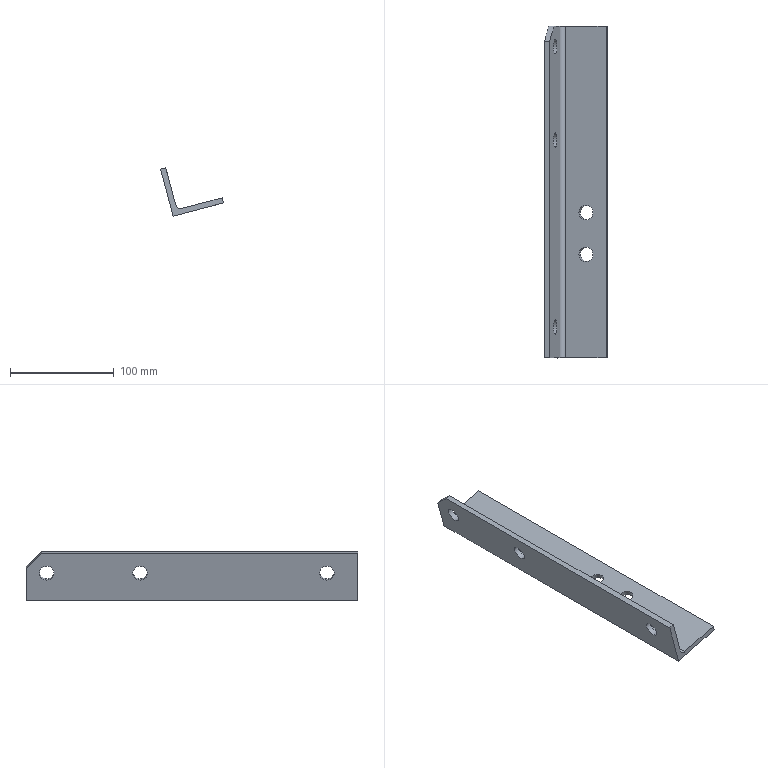Part | NX | features solid 2 | 1 solid | 15 faces | box 60.461 x 320 x 46.693 mm | volume 144506 mm3 | plane 9 | cylinder 6 | commonest cylinder face diameters 14 x5 10 x1
STEP:
#1=CARTESIAN_POINT('',(712.611,850.,-13.897));
#2=VERTEX_POINT('',#1);
#3=CARTESIAN_POINT('',(719.373,850.,-12.085));
#4=DIRECTION('',(-0.2588,0.,0.9659));
#5=DIRECTION('',(-0.9659,0.,-0.2588));
#6=AXIS2_PLACEMENT_3D('',#3,#4,#5);
#7=CIRCLE('',#6,7.);
#8=EDGE_CURVE('',#2,#2,#7,.T.);
#9=ORIENTED_EDGE('',*,*,#8,.F.);
#10=EDGE_LOOP('',(#9));
#11=FACE_BOUND('',#10,.T.);
#12=CARTESIAN_POINT('',(712.611,890.,-13.897));
#13=VERTEX_POINT('',#12);
#14=CARTESIAN_POINT('',(719.373,890.,-12.085));
#15=DIRECTION('',(-0.2588,0.,0.9659));
#16=DIRECTION('',(-0.9659,0.,-0.2588));
#17=AXIS2_PLACEMENT_3D('',#14,#15,#16);
#18=CIRCLE('',#17,7.);
#19=EDGE_CURVE('',#13,#13,#18,.T.);
#20=ORIENTED_EDGE('',*,*,#19,.F.);
#21=EDGE_LOOP('',(#20));
#22=FACE_BOUND('',#21,.T.);
#23=CARTESIAN_POINT('',(700.054,1070.,-17.261));
#24=VERTEX_POINT('',#23);
#25=CARTESIAN_POINT('',(700.054,750.,-17.261));
#26=VERTEX_POINT('',#25);
#27=CARTESIAN_POINT('',(700.054,775.,-17.261));
#28=DIRECTION('',(0.,1.,0.));
#29=VECTOR('',#28,1000.);
#30=LINE('',#27,#29);
#31=EDGE_CURVE('',#24,#26,#30,.F.);
#32=ORIENTED_EDGE('',*,*,#31,.T.);
#33=CARTESIAN_POINT('',(738.691,750.,-6.909));
#34=VERTEX_POINT('',#33);
#35=CARTESIAN_POINT('',(738.691,750.,-6.909));
#36=DIRECTION('',(0.9659,0.,0.2588));
#37=VECTOR('',#36,1000.);
#38=LINE('',#35,#37);
#39=EDGE_CURVE('',#26,#34,#38,.T.);
#40=ORIENTED_EDGE('',*,*,#39,.T.);
#41=CARTESIAN_POINT('',(738.691,1070.,-6.909));
#42=VERTEX_POINT('',#41);
#43=CARTESIAN_POINT('',(738.691,894.636,-6.909));
#44=DIRECTION('',(0.,1.,0.));
#45=VECTOR('',#44,1000.);
#46=LINE('',#43,#45);
#47=EDGE_CURVE('',#34,#42,#46,.T.);
#48=ORIENTED_EDGE('',*,*,#47,.T.);
#49=CARTESIAN_POINT('',(738.691,1070.,-6.909));
#50=DIRECTION('',(0.9659,0.,0.2588));
#51=VECTOR('',#50,1000.);
#52=LINE('',#49,#51);
#53=EDGE_CURVE('',#24,#42,#52,.T.);
#54=ORIENTED_EDGE('',*,*,#53,.F.);
#55=EDGE_LOOP('',(#32,#40,#48,#54));
#56=FACE_BOUND('',#55,.T.);
#57=CARTESIAN_POINT('',(738.691,892.805,-6.909));
#58=DIRECTION('',(-0.2588,0.,0.9659));
#59=DIRECTION('',(0.,1.,0.));
#60=AXIS2_PLACEMENT_3D('',#57,#58,#59);
#61=PLANE('',#60);
#62=ADVANCED_FACE('',(#11,#22,#56),#61,.T.);
#63=CARTESIAN_POINT('',(713.905,850.,-18.726));
#64=VERTEX_POINT('',#63);
#65=CARTESIAN_POINT('',(720.667,850.,-16.915));
#66=DIRECTION('',(-0.2588,0.,0.9659));
#67=DIRECTION('',(-0.9659,0.,-0.2588));
#68=AXIS2_PLACEMENT_3D('',#65,#66,#67);
#69=CIRCLE('',#68,7.);
#70=EDGE_CURVE('',#64,#64,#69,.F.);
#71=ORIENTED_EDGE('',*,*,#70,.F.);
#72=EDGE_LOOP('',(#71));
#73=FACE_BOUND('',#72,.T.);
#74=CARTESIAN_POINT('',(713.905,890.,-18.726));
#75=VERTEX_POINT('',#74);
#76=CARTESIAN_POINT('',(720.667,890.,-16.915));
#77=DIRECTION('',(-0.2588,0.,0.9659));
#78=DIRECTION('',(-0.9659,0.,-0.2588));
#79=AXIS2_PLACEMENT_3D('',#76,#77,#78);
#80=CIRCLE('',#79,7.);
#81=EDGE_CURVE('',#75,#75,#80,.F.);
#82=ORIENTED_EDGE('',*,*,#81,.F.);
#83=EDGE_LOOP('',(#82));
#84=FACE_BOUND('',#83,.T.);
#85=CARTESIAN_POINT('',(739.985,750.,-11.738));
#86=VERTEX_POINT('',#85);
#87=CARTESIAN_POINT('',(739.985,1070.,-11.738));
#88=VERTEX_POINT('',#87);
#89=CARTESIAN_POINT('',(739.985,892.5,-11.738));
#90=DIRECTION('',(0.,1.,0.));
#91=VECTOR('',#90,1000.);
#92=LINE('',#89,#91);
#93=EDGE_CURVE('',#86,#88,#92,.T.);
#94=ORIENTED_EDGE('',*,*,#93,.F.);
#95=CARTESIAN_POINT('',(691.689,750.,-24.679));
#96=VERTEX_POINT('',#95);
#97=CARTESIAN_POINT('',(696.519,750.,-23.385));
#98=DIRECTION('',(-0.9659,0.,-0.2588));
#99=VECTOR('',#98,1000.);
#100=LINE('',#97,#99);
#101=EDGE_CURVE('',#86,#96,#100,.T.);
#102=ORIENTED_EDGE('',*,*,#101,.T.);
#103=CARTESIAN_POINT('',(691.689,1070.,-24.679));
#104=VERTEX_POINT('',#103);
#105=CARTESIAN_POINT('',(691.689,894.636,-24.679));
#106=DIRECTION('',(0.,1.,0.));
#107=VECTOR('',#106,1000.);
#108=LINE('',#105,#107);
#109=EDGE_CURVE('',#96,#104,#108,.T.);
#110=ORIENTED_EDGE('',*,*,#109,.T.);
#111=CARTESIAN_POINT('',(696.519,1070.,-23.385));
#112=DIRECTION('',(-0.9659,0.,-0.2588));
#113=VECTOR('',#112,1000.);
#114=LINE('',#111,#113);
#115=EDGE_CURVE('',#88,#104,#114,.T.);
#116=ORIENTED_EDGE('',*,*,#115,.F.);
#117=EDGE_LOOP('',(#94,#102,#110,#116));
#118=FACE_BOUND('',#117,.T.);
#119=CARTESIAN_POINT('',(696.519,892.5,-23.385));
#120=DIRECTION('',(0.2588,0.,-0.9659));
#121=DIRECTION('',(0.,-1.,0.));
#122=AXIS2_PLACEMENT_3D('',#119,#120,#121);
#123=PLANE('',#122);
#124=ADVANCED_FACE('',(#73,#84,#118),#123,.T.);
#125=CARTESIAN_POINT('',(687.719,1050.,9.456));
#126=VERTEX_POINT('',#125);
#127=CARTESIAN_POINT('',(689.531,1050.,2.695));
#128=DIRECTION('',(0.9659,0.,0.2588));
#129=DIRECTION('',(-0.2588,0.,0.9659));
#130=AXIS2_PLACEMENT_3D('',#127,#128,#129);
#131=CIRCLE('',#130,7.);
#132=EDGE_CURVE('',#126,#126,#131,.F.);
#133=ORIENTED_EDGE('',*,*,#132,.T.);
#134=EDGE_LOOP('',(#133));
#135=FACE_BOUND('',#134,.T.);
#136=CARTESIAN_POINT('',(691.342,960.,-4.067));
#137=VERTEX_POINT('',#136);
#138=CARTESIAN_POINT('',(689.531,960.,2.695));
#139=DIRECTION('',(-0.9659,0.,-0.2588));
#140=DIRECTION('',(0.2588,0.,-0.9659));
#141=AXIS2_PLACEMENT_3D('',#138,#139,#140);
#142=CIRCLE('',#141,7.);
#143=EDGE_CURVE('',#137,#137,#142,.F.);
#144=ORIENTED_EDGE('',*,*,#143,.F.);
#145=EDGE_LOOP('',(#144));
#146=FACE_BOUND('',#145,.T.);
#147=CARTESIAN_POINT('',(691.342,780.,-4.067));
#148=VERTEX_POINT('',#147);
#149=CARTESIAN_POINT('',(689.531,780.,2.695));
#150=DIRECTION('',(-0.9659,0.,-0.2588));
#151=DIRECTION('',(0.2588,0.,-0.9659));
#152=AXIS2_PLACEMENT_3D('',#149,#150,#151);
#153=CIRCLE('',#152,7.);
#154=EDGE_CURVE('',#148,#148,#153,.F.);
#155=ORIENTED_EDGE('',*,*,#154,.F.);
#156=EDGE_LOOP('',(#155));
#157=FACE_BOUND('',#156,.T.);
#158=CARTESIAN_POINT('',(684.354,750.,22.013));
#159=VERTEX_POINT('',#158);
#160=CARTESIAN_POINT('',(684.354,1055.,22.013));
#161=VERTEX_POINT('',#160);
#162=CARTESIAN_POINT('',(684.354,894.636,22.013));
#163=DIRECTION('',(0.,1.,0.));
#164=VECTOR('',#163,1000.);
#165=LINE('',#162,#164);
#166=EDGE_CURVE('',#159,#161,#165,.T.);
#167=ORIENTED_EDGE('',*,*,#166,.F.);
#168=CARTESIAN_POINT('',(693.93,750.,-13.726));
#169=VERTEX_POINT('',#168);
#170=CARTESIAN_POINT('',(687.46,750.,10.422));
#171=DIRECTION('',(0.2588,0.,-0.9659));
#172=VECTOR('',#171,1000.);
#173=LINE('',#170,#172);
#174=EDGE_CURVE('',#159,#169,#173,.T.);
#175=ORIENTED_EDGE('',*,*,#174,.T.);
#176=CARTESIAN_POINT('',(693.93,1070.,-13.726));
#177=VERTEX_POINT('',#176);
#178=CARTESIAN_POINT('',(693.93,1109.813,-13.726));
#179=DIRECTION('',(0.,1.,0.));
#180=VECTOR('',#179,1000.);
#181=LINE('',#178,#180);
#182=EDGE_CURVE('',#169,#177,#181,.T.);
#183=ORIENTED_EDGE('',*,*,#182,.T.);
#184=CARTESIAN_POINT('',(688.236,1070.,7.525));
#185=VERTEX_POINT('',#184);
#186=CARTESIAN_POINT('',(687.46,1070.,10.422));
#187=DIRECTION('',(0.2588,0.,-0.9659));
#188=VECTOR('',#187,1000.);
#189=LINE('',#186,#188);
#190=EDGE_CURVE('',#185,#177,#189,.T.);
#191=ORIENTED_EDGE('',*,*,#190,.F.);
#192=CARTESIAN_POINT('',(665.154,980.818,93.668));
#193=DIRECTION('',(-0.183,-0.7071,0.683));
#194=VECTOR('',#193,1000.);
#195=LINE('',#192,#194);
#196=EDGE_CURVE('',#185,#161,#195,.T.);
#197=ORIENTED_EDGE('',*,*,#196,.T.);
#198=EDGE_LOOP('',(#167,#175,#183,#191,#197));
#199=FACE_BOUND('',#198,.T.);
#200=CARTESIAN_POINT('',(687.46,894.636,10.422));
#201=DIRECTION('',(0.9659,0.,0.2588));
#202=DIRECTION('',(0.2588,0.,-0.9659));
#203=AXIS2_PLACEMENT_3D('',#200,#201,#202);
#204=PLANE('',#203);
#205=ADVANCED_FACE('',(#135,#146,#157,#199),#204,.T.);
#206=CARTESIAN_POINT('',(686.513,1050.,-5.361));
#207=VERTEX_POINT('',#206);
#208=CARTESIAN_POINT('',(684.701,1050.,1.401));
#209=DIRECTION('',(-0.9659,0.,-0.2588));
#210=DIRECTION('',(0.2588,0.,-0.9659));
#211=AXIS2_PLACEMENT_3D('',#208,#209,#210);
#212=CIRCLE('',#211,7.);
#213=EDGE_CURVE('',#207,#207,#212,.T.);
#214=ORIENTED_EDGE('',*,*,#213,.F.);
#215=EDGE_LOOP('',(#214));
#216=FACE_BOUND('',#215,.T.);
#217=CARTESIAN_POINT('',(682.889,960.,8.162));
#218=VERTEX_POINT('',#217);
#219=CARTESIAN_POINT('',(684.701,960.,1.401));
#220=DIRECTION('',(0.9659,0.,0.2588));
#221=DIRECTION('',(-0.2588,0.,0.9659));
#222=AXIS2_PLACEMENT_3D('',#219,#220,#221);
#223=CIRCLE('',#222,7.);
#224=EDGE_CURVE('',#218,#218,#223,.F.);
#225=ORIENTED_EDGE('',*,*,#224,.F.);
#226=EDGE_LOOP('',(#225));
#227=FACE_BOUND('',#226,.T.);
#228=CARTESIAN_POINT('',(682.889,780.,8.162));
#229=VERTEX_POINT('',#228);
#230=CARTESIAN_POINT('',(684.701,780.,1.401));
#231=DIRECTION('',(0.9659,0.,0.2588));
#232=DIRECTION('',(-0.2588,0.,0.9659));
#233=AXIS2_PLACEMENT_3D('',#230,#231,#232);
#234=CIRCLE('',#233,7.);
#235=EDGE_CURVE('',#229,#229,#234,.F.);
#236=ORIENTED_EDGE('',*,*,#235,.F.);
#237=EDGE_LOOP('',(#236));
#238=FACE_BOUND('',#237,.T.);
#239=ORIENTED_EDGE('',*,*,#109,.F.);
#240=CARTESIAN_POINT('',(679.525,750.,20.719));
#241=VERTEX_POINT('',#240);
#242=CARTESIAN_POINT('',(682.63,750.,9.128));
#243=DIRECTION('',(-0.2588,0.,0.9659));
#244=VECTOR('',#243,1000.);
#245=LINE('',#242,#244);
#246=EDGE_CURVE('',#96,#241,#245,.T.);
#247=ORIENTED_EDGE('',*,*,#246,.T.);
#248=CARTESIAN_POINT('',(679.525,1055.,20.719));
#249=VERTEX_POINT('',#248);
#250=CARTESIAN_POINT('',(679.525,894.636,20.719));
#251=DIRECTION('',(0.,1.,0.));
#252=VECTOR('',#251,1000.);
#253=LINE('',#250,#252);
#254=EDGE_CURVE('',#241,#249,#253,.T.);
#255=ORIENTED_EDGE('',*,*,#254,.T.);
#256=CARTESIAN_POINT('',(683.407,1070.,6.23));
#257=VERTEX_POINT('',#256);
#258=CARTESIAN_POINT('',(660.325,980.818,92.374));
#259=DIRECTION('',(0.183,0.7071,-0.683));
#260=VECTOR('',#259,1000.);
#261=LINE('',#258,#260);
#262=EDGE_CURVE('',#249,#257,#261,.T.);
#263=ORIENTED_EDGE('',*,*,#262,.T.);
#264=CARTESIAN_POINT('',(682.63,1070.,9.128));
#265=DIRECTION('',(-0.2588,0.,0.9659));
#266=VECTOR('',#265,1000.);
#267=LINE('',#264,#266);
#268=EDGE_CURVE('',#104,#257,#267,.T.);
#269=ORIENTED_EDGE('',*,*,#268,.F.);
#270=EDGE_LOOP('',(#239,#247,#255,#263,#269));
#271=FACE_BOUND('',#270,.T.);
#272=CARTESIAN_POINT('',(682.63,894.636,9.128));
#273=DIRECTION('',(-0.9659,0.,-0.2588));
#274=DIRECTION('',(-0.2588,0.,0.9659));
#275=AXIS2_PLACEMENT_3D('',#272,#273,#274);
#276=PLANE('',#275);
#277=ADVANCED_FACE('',(#216,#227,#238,#271),#276,.T.);
#278=ORIENTED_EDGE('',*,*,#254,.F.);
#279=CARTESIAN_POINT('',(689.184,750.,23.308));
#280=DIRECTION('',(0.9659,0.,0.2588));
#281=VECTOR('',#280,1000.);
#282=LINE('',#279,#281);
#283=EDGE_CURVE('',#241,#159,#282,.T.);
#284=ORIENTED_EDGE('',*,*,#283,.T.);
#285=ORIENTED_EDGE('',*,*,#166,.T.);
#286=CARTESIAN_POINT('',(679.525,1055.,20.719));
#287=DIRECTION('',(-0.9659,0.,-0.2588));
#288=VECTOR('',#287,1000.);
#289=LINE('',#286,#288);
#290=EDGE_CURVE('',#161,#249,#289,.T.);
#291=ORIENTED_EDGE('',*,*,#290,.T.);
#292=EDGE_LOOP('',(#278,#284,#285,#291));
#293=FACE_BOUND('',#292,.T.);
#294=CARTESIAN_POINT('',(689.184,894.636,23.308));
#295=DIRECTION('',(-0.2588,0.,0.9659));
#296=DIRECTION('',(0.,1.,0.));
#297=AXIS2_PLACEMENT_3D('',#294,#295,#296);
#298=PLANE('',#297);
#299=ADVANCED_FACE('',(#293),#298,.T.);
#300=CARTESIAN_POINT('',(698.76,750.,-12.432));
#301=DIRECTION('',(0.,-1.,0.));
#302=DIRECTION('',(1.,0.,0.));
#303=AXIS2_PLACEMENT_3D('',#300,#301,#302);
#304=CIRCLE('',#303,5.);
#305=EDGE_CURVE('',#26,#169,#304,.F.);
#306=ORIENTED_EDGE('',*,*,#305,.F.);
#307=ORIENTED_EDGE('',*,*,#31,.F.);
#308=CARTESIAN_POINT('',(698.76,1070.,-12.432));
#309=DIRECTION('',(0.,-1.,0.));
#310=DIRECTION('',(0.1736,0.,0.9848));
#311=AXIS2_PLACEMENT_3D('',#308,#309,#310);
#312=CIRCLE('',#311,5.);
#313=EDGE_CURVE('',#24,#177,#312,.F.);
#314=ORIENTED_EDGE('',*,*,#313,.T.);
#315=ORIENTED_EDGE('',*,*,#182,.F.);
#316=EDGE_LOOP('',(#306,#307,#314,#315));
#317=FACE_BOUND('',#316,.T.);
#318=CARTESIAN_POINT('',(698.76,894.636,-12.432));
#319=DIRECTION('',(0.,-1.,0.));
#320=DIRECTION('',(0.2588,0.,-0.9659));
#321=AXIS2_PLACEMENT_3D('',#318,#319,#320);
#322=CYLINDRICAL_SURFACE('',#321,5.);
#323=ADVANCED_FACE('',(#317),#322,.F.);
#324=ORIENTED_EDGE('',*,*,#47,.F.);
#325=CARTESIAN_POINT('',(730.927,750.,22.069));
#326=DIRECTION('',(0.2588,0.,-0.9659));
#327=VECTOR('',#326,1000.);
#328=LINE('',#325,#327);
#329=EDGE_CURVE('',#34,#86,#328,.T.);
#330=ORIENTED_EDGE('',*,*,#329,.T.);
#331=ORIENTED_EDGE('',*,*,#93,.T.);
#332=CARTESIAN_POINT('',(730.927,1070.,22.069));
#333=DIRECTION('',(0.2588,0.,-0.9659));
#334=VECTOR('',#333,1000.);
#335=LINE('',#332,#334);
#336=EDGE_CURVE('',#42,#88,#335,.T.);
#337=ORIENTED_EDGE('',*,*,#336,.F.);
#338=EDGE_LOOP('',(#324,#330,#331,#337));
#339=FACE_BOUND('',#338,.T.);
#340=CARTESIAN_POINT('',(730.927,894.636,22.069));
#341=DIRECTION('',(0.9659,0.,0.2588));
#342=DIRECTION('',(0.2588,0.,-0.9659));
#343=AXIS2_PLACEMENT_3D('',#340,#341,#342);
#344=PLANE('',#343);
#345=ADVANCED_FACE('',(#339),#344,.T.);
#346=ORIENTED_EDGE('',*,*,#143,.T.);
#347=EDGE_LOOP('',(#346));
#348=FACE_BOUND('',#347,.T.);
#349=ORIENTED_EDGE('',*,*,#224,.T.);
#350=EDGE_LOOP('',(#349));
#351=FACE_BOUND('',#350,.T.);
#352=CARTESIAN_POINT('',(713.679,960.,9.165));
#353=DIRECTION('',(-0.9659,0.,-0.2588));
#354=DIRECTION('',(0.,1.,0.));
#355=AXIS2_PLACEMENT_3D('',#352,#353,#354);
#356=CYLINDRICAL_SURFACE('',#355,7.);
#357=ADVANCED_FACE('',(#348,#351),#356,.F.);
#358=ORIENTED_EDGE('',*,*,#268,.T.);
#359=CARTESIAN_POINT('',(688.236,1070.,7.525));
#360=DIRECTION('',(0.9659,0.,0.2588));
#361=VECTOR('',#360,1000.);
#362=LINE('',#359,#361);
#363=EDGE_CURVE('',#257,#185,#362,.T.);
#364=ORIENTED_EDGE('',*,*,#363,.T.);
#365=ORIENTED_EDGE('',*,*,#190,.T.);
#366=ORIENTED_EDGE('',*,*,#313,.F.);
#367=ORIENTED_EDGE('',*,*,#53,.T.);
#368=ORIENTED_EDGE('',*,*,#336,.T.);
#369=ORIENTED_EDGE('',*,*,#115,.T.);
#370=EDGE_LOOP('',(#358,#364,#365,#366,#367,#368,#369));
#371=FACE_BOUND('',#370,.T.);
#372=CARTESIAN_POINT('',(103.71,1070.,-64.317));
#373=DIRECTION('',(0.,-1.,0.));
#374=DIRECTION('',(0.1736,0.,0.9848));
#375=AXIS2_PLACEMENT_3D('',#372,#373,#374);
#376=PLANE('',#375);
#377=ADVANCED_FACE('',(#371),#376,.F.);
#378=ORIENTED_EDGE('',*,*,#154,.T.);
#379=EDGE_LOOP('',(#378));
#380=FACE_BOUND('',#379,.T.);
#381=ORIENTED_EDGE('',*,*,#235,.T.);
#382=EDGE_LOOP('',(#381));
#383=FACE_BOUND('',#382,.T.);
#384=CARTESIAN_POINT('',(713.679,780.,9.165));
#385=DIRECTION('',(-0.9659,0.,-0.2588));
#386=DIRECTION('',(0.,1.,0.));
#387=AXIS2_PLACEMENT_3D('',#384,#385,#386);
#388=CYLINDRICAL_SURFACE('',#387,7.);
#389=ADVANCED_FACE('',(#380,#383),#388,.F.);
#390=ORIENTED_EDGE('',*,*,#132,.F.);
#391=EDGE_LOOP('',(#390));
#392=FACE_BOUND('',#391,.T.);
#393=ORIENTED_EDGE('',*,*,#213,.T.);
#394=EDGE_LOOP('',(#393));
#395=FACE_BOUND('',#394,.T.);
#396=CARTESIAN_POINT('',(713.679,1050.,9.165));
#397=DIRECTION('',(-0.9659,0.,-0.2588));
#398=DIRECTION('',(0.,1.,0.));
#399=AXIS2_PLACEMENT_3D('',#396,#397,#398);
#400=CYLINDRICAL_SURFACE('',#399,7.);
#401=ADVANCED_FACE('',(#392,#395),#400,.F.);
#402=ORIENTED_EDGE('',*,*,#262,.F.);
#403=ORIENTED_EDGE('',*,*,#290,.F.);
#404=ORIENTED_EDGE('',*,*,#196,.F.);
#405=ORIENTED_EDGE('',*,*,#363,.F.);
#406=EDGE_LOOP('',(#402,#403,#404,#405));
#407=FACE_BOUND('',#406,.T.);
#408=CARTESIAN_POINT('',(124.906,1070.,-143.419));
#409=DIRECTION('',(-0.183,0.7071,0.683));
#410=DIRECTION('',(-0.1287,0.6715,-0.7297));
#411=AXIS2_PLACEMENT_3D('',#408,#409,#410);
#412=PLANE('',#411);
#413=ADVANCED_FACE('',(#407),#412,.T.);
#414=ORIENTED_EDGE('',*,*,#81,.T.);
#415=EDGE_LOOP('',(#414));
#416=FACE_BOUND('',#415,.T.);
#417=ORIENTED_EDGE('',*,*,#19,.T.);
#418=EDGE_LOOP('',(#417));
#419=FACE_BOUND('',#418,.T.);
#420=CARTESIAN_POINT('',(732.314,890.,-60.381));
#421=DIRECTION('',(-0.2588,0.,0.9659));
#422=DIRECTION('',(-0.9659,0.,-0.2588));
#423=AXIS2_PLACEMENT_3D('',#420,#421,#422);
#424=CYLINDRICAL_SURFACE('',#423,7.);
#425=ADVANCED_FACE('',(#416,#419),#424,.F.);
#426=ORIENTED_EDGE('',*,*,#70,.T.);
#427=EDGE_LOOP('',(#426));
#428=FACE_BOUND('',#427,.T.);
#429=ORIENTED_EDGE('',*,*,#8,.T.);
#430=EDGE_LOOP('',(#429));
#431=FACE_BOUND('',#430,.T.);
#432=CARTESIAN_POINT('',(732.314,850.,-60.381));
#433=DIRECTION('',(-0.2588,0.,0.9659));
#434=DIRECTION('',(-0.9659,0.,-0.2588));
#435=AXIS2_PLACEMENT_3D('',#432,#433,#434);
#436=CYLINDRICAL_SURFACE('',#435,7.);
#437=ADVANCED_FACE('',(#428,#431),#436,.F.);
#438=ORIENTED_EDGE('',*,*,#283,.F.);
#439=ORIENTED_EDGE('',*,*,#246,.F.);
#440=ORIENTED_EDGE('',*,*,#101,.F.);
#441=ORIENTED_EDGE('',*,*,#329,.F.);
#442=ORIENTED_EDGE('',*,*,#39,.F.);
#443=ORIENTED_EDGE('',*,*,#305,.T.);
#444=ORIENTED_EDGE('',*,*,#174,.F.);
#445=EDGE_LOOP('',(#438,#439,#440,#441,#442,#443,#444));
#446=FACE_BOUND('',#445,.T.);
#447=CARTESIAN_POINT('',(711.696,750.,-8.577));
#448=DIRECTION('',(0.,-1.,0.));
#449=DIRECTION('',(1.,0.,0.));
#450=AXIS2_PLACEMENT_3D('',#447,#448,#449);
#451=PLANE('',#450);
#452=ADVANCED_FACE('',(#446),#451,.T.);
#453=CLOSED_SHELL('',(#62,#124,#205,#277,#299,#323,#345,#357,#377,#389,#401,#413,#425,#437,#452));
#454=MANIFOLD_SOLID_BREP('',#453);
#455=(LENGTH_UNIT()NAMED_UNIT(*)SI_UNIT(.MILLI.,.METRE.));
#456=UNCERTAINTY_MEASURE_WITH_UNIT(LENGTH_MEASURE(0.00001),#455,'','');
#457=(NAMED_UNIT(*)PLANE_ANGLE_UNIT()SI_UNIT($,.RADIAN.));
#458=(NAMED_UNIT(*)SI_UNIT($,.STERADIAN.)SOLID_ANGLE_UNIT());
#459=(GEOMETRIC_REPRESENTATION_CONTEXT(3)GLOBAL_UNCERTAINTY_ASSIGNED_CONTEXT((#456))GLOBAL_UNIT_ASSIGNED_CONTEXT((#455,#457,#458))REPRESENTATION_CONTEXT('',''));
#460=ADVANCED_BREP_SHAPE_REPRESENTATION('',(#454),#459);